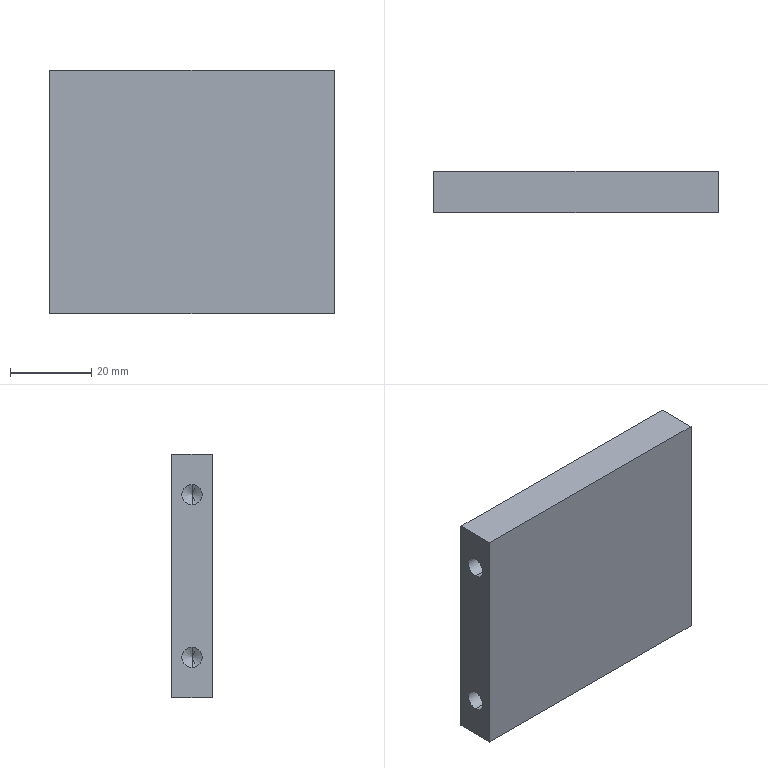Part | STEP file | Tube support mounting bracket upright plate | 1 solid | 22 faces | box 70 x 10 x 60 mm | volume 40154 mm3 | cylinder 8 | cone 8 | plane 6 | commonest cylinder face diameters 5 x8
STEP:
#1=CARTESIAN_POINT('',(0.,0.,0.));
#2=DIRECTION('',(0.,0.,1.));
#3=DIRECTION('',(1.,0.,0.));
#4=AXIS2_PLACEMENT_3D('',#1,#2,#3);
#5=CARTESIAN_POINT('',(-12.,0.,22.5));
#6=VERTEX_POINT('',#5);
#7=CARTESIAN_POINT('',(-35.,0.,22.5));
#8=VERTEX_POINT('',#7);
#9=CARTESIAN_POINT('',(-35.,0.,22.5));
#10=DIRECTION('',(-1.,0.,0.));
#11=VECTOR('',#10,1.);
#12=LINE('',#9,#11);
#13=CARTESIAN_POINT('',(-35.,0.,20.));
#14=DIRECTION('',(-1.,0.,0.));
#15=DIRECTION('',(0.,0.,1.));
#16=AXIS2_PLACEMENT_3D('',#13,#14,#15);
#17=CYLINDRICAL_SURFACE('',#16,2.5);
#18=CARTESIAN_POINT('',(6.283,0.));
#19=DIRECTION('',(0.,1.));
#20=VECTOR('',#19,1.);
#21=LINE('',#18,#20);
#22=(GEOMETRIC_REPRESENTATION_CONTEXT(2)PARAMETRIC_REPRESENTATION_CONTEXT()REPRESENTATION_CONTEXT('',''));
#23=DEFINITIONAL_REPRESENTATION('',(#21),#22);
#24=PCURVE('',#17,#23);
#25=CARTESIAN_POINT('',(-35.,0.,20.));
#26=DIRECTION('',(-1.,0.,0.));
#27=DIRECTION('',(0.,0.,1.));
#28=AXIS2_PLACEMENT_3D('',#25,#26,#27);
#29=CYLINDRICAL_SURFACE('',#28,2.5);
#30=CARTESIAN_POINT('',(0.,0.));
#31=DIRECTION('',(0.,1.));
#32=VECTOR('',#31,1.);
#33=LINE('',#30,#32);
#34=(GEOMETRIC_REPRESENTATION_CONTEXT(2)PARAMETRIC_REPRESENTATION_CONTEXT()REPRESENTATION_CONTEXT('',''));
#35=DEFINITIONAL_REPRESENTATION('',(#33),#34);
#36=PCURVE('',#29,#35);
#37=SURFACE_CURVE('',#12,(#24,#36),.PCURVE_S1.);
#38=EDGE_CURVE('',#6,#8,#37,.T.);
#39=ORIENTED_EDGE('',*,*,#38,.T.);
#40=CARTESIAN_POINT('',(-35.,0.,17.5));
#41=VERTEX_POINT('',#40);
#42=CARTESIAN_POINT('',(-35.,0.,20.));
#43=DIRECTION('',(-1.,0.,0.));
#44=DIRECTION('',(0.,0.,1.));
#45=AXIS2_PLACEMENT_3D('',#42,#43,#44);
#46=CIRCLE('',#45,2.5);
#47=CARTESIAN_POINT('',(0.,0.));
#48=DIRECTION('',(1.,0.));
#49=VECTOR('',#48,1.);
#50=LINE('',#47,#49);
#51=(GEOMETRIC_REPRESENTATION_CONTEXT(2)PARAMETRIC_REPRESENTATION_CONTEXT()REPRESENTATION_CONTEXT('',''));
#52=DEFINITIONAL_REPRESENTATION('',(#50),#51);
#53=PCURVE('',#17,#52);
#54=CARTESIAN_POINT('',(-35.,5.,30.));
#55=DIRECTION('',(1.,0.,0.));
#56=DIRECTION('',(0.,0.,-1.));
#57=AXIS2_PLACEMENT_3D('',#54,#55,#56);
#58=PLANE('',#57);
#59=CARTESIAN_POINT('',(7.5,-5.));
#60=CARTESIAN_POINT('',(7.5,-0.6699));
#61=CARTESIAN_POINT('',(11.25,-2.835));
#62=CARTESIAN_POINT('',(15.,-5.));
#63=CARTESIAN_POINT('',(11.25,-7.165));
#64=CARTESIAN_POINT('',(7.5,-9.33));
#65=CARTESIAN_POINT('',(7.5,-5.));
#66=(BOUNDED_CURVE()B_SPLINE_CURVE(2,(#59,#60,#61,#62,#63,#64,#65),.UNSPECIFIED.,.T.,.F.)B_SPLINE_CURVE_WITH_KNOTS((1,2,2,2,2,1),(-2.094,0.,2.094,4.189,6.283,8.378),.UNSPECIFIED.)CURVE()GEOMETRIC_REPRESENTATION_ITEM()RATIONAL_B_SPLINE_CURVE((1.,0.5,1.,0.5,1.,0.5,1.))REPRESENTATION_ITEM(''));
#67=(GEOMETRIC_REPRESENTATION_CONTEXT(2)PARAMETRIC_REPRESENTATION_CONTEXT()REPRESENTATION_CONTEXT('',''));
#68=DEFINITIONAL_REPRESENTATION('',(#66),#67);
#69=PCURVE('',#58,#68);
#70=SURFACE_CURVE('',#46,(#53,#69),.PCURVE_S1.);
#71=EDGE_CURVE('',#41,#8,#70,.T.);
#72=ORIENTED_EDGE('',*,*,#71,.F.);
#73=CARTESIAN_POINT('',(-12.,0.,17.5));
#74=VERTEX_POINT('',#73);
#75=CARTESIAN_POINT('',(-35.,0.,17.5));
#76=DIRECTION('',(-1.,0.,0.));
#77=VECTOR('',#76,1.);
#78=LINE('',#75,#77);
#79=CARTESIAN_POINT('',(3.142,0.));
#80=DIRECTION('',(0.,1.));
#81=VECTOR('',#80,1.);
#82=LINE('',#79,#81);
#83=(GEOMETRIC_REPRESENTATION_CONTEXT(2)PARAMETRIC_REPRESENTATION_CONTEXT()REPRESENTATION_CONTEXT('',''));
#84=DEFINITIONAL_REPRESENTATION('',(#82),#83);
#85=PCURVE('',#17,#84);
#86=CARTESIAN_POINT('',(3.142,0.));
#87=DIRECTION('',(0.,1.));
#88=VECTOR('',#87,1.);
#89=LINE('',#86,#88);
#90=(GEOMETRIC_REPRESENTATION_CONTEXT(2)PARAMETRIC_REPRESENTATION_CONTEXT()REPRESENTATION_CONTEXT('',''));
#91=DEFINITIONAL_REPRESENTATION('',(#89),#90);
#92=PCURVE('',#29,#91);
#93=SURFACE_CURVE('',#78,(#85,#92),.PCURVE_S1.);
#94=EDGE_CURVE('',#74,#41,#93,.T.);
#95=ORIENTED_EDGE('',*,*,#94,.F.);
#96=CARTESIAN_POINT('',(-12.,0.,20.));
#97=DIRECTION('',(-1.,0.,0.));
#98=DIRECTION('',(0.,0.,1.));
#99=AXIS2_PLACEMENT_3D('',#96,#97,#98);
#100=CIRCLE('',#99,2.5);
#101=CARTESIAN_POINT('',(0.,-23.));
#102=DIRECTION('',(1.,0.));
#103=VECTOR('',#102,1.);
#104=LINE('',#101,#103);
#105=(GEOMETRIC_REPRESENTATION_CONTEXT(2)PARAMETRIC_REPRESENTATION_CONTEXT()REPRESENTATION_CONTEXT('',''));
#106=DEFINITIONAL_REPRESENTATION('',(#104),#105);
#107=PCURVE('',#17,#106);
#108=CARTESIAN_POINT('',(-12.,0.,20.));
#109=DIRECTION('',(-1.,0.,0.));
#110=DIRECTION('',(0.,0.,1.));
#111=AXIS2_PLACEMENT_3D('',#108,#109,#110);
#112=CONICAL_SURFACE('',#111,2.5,1.03);
#113=CARTESIAN_POINT('',(0.,0.));
#114=DIRECTION('',(1.,0.));
#115=VECTOR('',#114,1.);
#116=LINE('',#113,#115);
#117=(GEOMETRIC_REPRESENTATION_CONTEXT(2)PARAMETRIC_REPRESENTATION_CONTEXT()REPRESENTATION_CONTEXT('',''));
#118=DEFINITIONAL_REPRESENTATION('',(#116),#117);
#119=PCURVE('',#112,#118);
#120=SURFACE_CURVE('',#100,(#107,#119),.PCURVE_S1.);
#121=EDGE_CURVE('',#74,#6,#120,.T.);
#122=ORIENTED_EDGE('',*,*,#121,.T.);
#123=EDGE_LOOP('',(#39,#72,#95,#122));
#124=FACE_BOUND('',#123,.F.);
#125=ADVANCED_FACE('',(#124),#17,.F.);
#126=ORIENTED_EDGE('',*,*,#121,.F.);
#127=CARTESIAN_POINT('',(-10.498,0.,20.));
#128=VERTEX_POINT('',#127);
#129=CARTESIAN_POINT('',(-12.,0.,17.5));
#130=DIRECTION('',(-0.515,0.,-0.8572));
#131=VECTOR('',#130,1.);
#132=LINE('',#129,#131);
#133=CARTESIAN_POINT('',(3.142,0.));
#134=DIRECTION('',(0.,1.));
#135=VECTOR('',#134,1.);
#136=LINE('',#133,#135);
#137=(GEOMETRIC_REPRESENTATION_CONTEXT(2)PARAMETRIC_REPRESENTATION_CONTEXT()REPRESENTATION_CONTEXT('',''));
#138=DEFINITIONAL_REPRESENTATION('',(#136),#137);
#139=PCURVE('',#112,#138);
#140=CARTESIAN_POINT('',(-12.,0.,20.));
#141=DIRECTION('',(-1.,0.,0.));
#142=DIRECTION('',(0.,0.,1.));
#143=AXIS2_PLACEMENT_3D('',#140,#141,#142);
#144=CONICAL_SURFACE('',#143,2.5,1.03);
#145=CARTESIAN_POINT('',(3.142,0.));
#146=DIRECTION('',(0.,1.));
#147=VECTOR('',#146,1.);
#148=LINE('',#145,#147);
#149=(GEOMETRIC_REPRESENTATION_CONTEXT(2)PARAMETRIC_REPRESENTATION_CONTEXT()REPRESENTATION_CONTEXT('',''));
#150=DEFINITIONAL_REPRESENTATION('',(#148),#149);
#151=PCURVE('',#144,#150);
#152=SURFACE_CURVE('',#132,(#139,#151),.PCURVE_S1.);
#153=EDGE_CURVE('',#128,#74,#152,.T.);
#154=ORIENTED_EDGE('',*,*,#153,.F.);
#155=CARTESIAN_POINT('',(-12.,0.,22.5));
#156=DIRECTION('',(-0.515,0.,0.8572));
#157=VECTOR('',#156,1.);
#158=LINE('',#155,#157);
#159=CARTESIAN_POINT('',(6.283,0.));
#160=DIRECTION('',(0.,1.));
#161=VECTOR('',#160,1.);
#162=LINE('',#159,#161);
#163=(GEOMETRIC_REPRESENTATION_CONTEXT(2)PARAMETRIC_REPRESENTATION_CONTEXT()REPRESENTATION_CONTEXT('',''));
#164=DEFINITIONAL_REPRESENTATION('',(#162),#163);
#165=PCURVE('',#112,#164);
#166=CARTESIAN_POINT('',(0.,0.));
#167=DIRECTION('',(0.,1.));
#168=VECTOR('',#167,1.);
#169=LINE('',#166,#168);
#170=(GEOMETRIC_REPRESENTATION_CONTEXT(2)PARAMETRIC_REPRESENTATION_CONTEXT()REPRESENTATION_CONTEXT('',''));
#171=DEFINITIONAL_REPRESENTATION('',(#169),#170);
#172=PCURVE('',#144,#171);
#173=SURFACE_CURVE('',#158,(#165,#172),.PCURVE_S1.);
#174=EDGE_CURVE('',#128,#6,#173,.T.);
#175=ORIENTED_EDGE('',*,*,#174,.T.);
#176=EDGE_LOOP('',(#126,#154,#175));
#177=FACE_BOUND('',#176,.F.);
#178=ADVANCED_FACE('',(#177),#112,.F.);
#179=CARTESIAN_POINT('',(-12.,0.,-17.5));
#180=VERTEX_POINT('',#179);
#181=CARTESIAN_POINT('',(-35.,0.,-17.5));
#182=VERTEX_POINT('',#181);
#183=CARTESIAN_POINT('',(-35.,0.,-17.5));
#184=DIRECTION('',(-1.,0.,0.));
#185=VECTOR('',#184,1.);
#186=LINE('',#183,#185);
#187=CARTESIAN_POINT('',(-35.,0.,-20.));
#188=DIRECTION('',(-1.,0.,0.));
#189=DIRECTION('',(0.,0.,1.));
#190=AXIS2_PLACEMENT_3D('',#187,#188,#189);
#191=CYLINDRICAL_SURFACE('',#190,2.5);
#192=CARTESIAN_POINT('',(6.283,0.));
#193=DIRECTION('',(0.,1.));
#194=VECTOR('',#193,1.);
#195=LINE('',#192,#194);
#196=(GEOMETRIC_REPRESENTATION_CONTEXT(2)PARAMETRIC_REPRESENTATION_CONTEXT()REPRESENTATION_CONTEXT('',''));
#197=DEFINITIONAL_REPRESENTATION('',(#195),#196);
#198=PCURVE('',#191,#197);
#199=CARTESIAN_POINT('',(-35.,0.,-20.));
#200=DIRECTION('',(-1.,0.,0.));
#201=DIRECTION('',(0.,0.,1.));
#202=AXIS2_PLACEMENT_3D('',#199,#200,#201);
#203=CYLINDRICAL_SURFACE('',#202,2.5);
#204=CARTESIAN_POINT('',(0.,0.));
#205=DIRECTION('',(0.,1.));
#206=VECTOR('',#205,1.);
#207=LINE('',#204,#206);
#208=(GEOMETRIC_REPRESENTATION_CONTEXT(2)PARAMETRIC_REPRESENTATION_CONTEXT()REPRESENTATION_CONTEXT('',''));
#209=DEFINITIONAL_REPRESENTATION('',(#207),#208);
#210=PCURVE('',#203,#209);
#211=SURFACE_CURVE('',#186,(#198,#210),.PCURVE_S1.);
#212=EDGE_CURVE('',#180,#182,#211,.T.);
#213=ORIENTED_EDGE('',*,*,#212,.T.);
#214=CARTESIAN_POINT('',(-35.,0.,-22.5));
#215=VERTEX_POINT('',#214);
#216=CARTESIAN_POINT('',(-35.,0.,-20.));
#217=DIRECTION('',(-1.,0.,0.));
#218=DIRECTION('',(0.,0.,1.));
#219=AXIS2_PLACEMENT_3D('',#216,#217,#218);
#220=CIRCLE('',#219,2.5);
#221=CARTESIAN_POINT('',(0.,0.));
#222=DIRECTION('',(1.,0.));
#223=VECTOR('',#222,1.);
#224=LINE('',#221,#223);
#225=(GEOMETRIC_REPRESENTATION_CONTEXT(2)PARAMETRIC_REPRESENTATION_CONTEXT()REPRESENTATION_CONTEXT('',''));
#226=DEFINITIONAL_REPRESENTATION('',(#224),#225);
#227=PCURVE('',#191,#226);
#228=CARTESIAN_POINT('',(47.5,-5.));
#229=CARTESIAN_POINT('',(47.5,-0.6699));
#230=CARTESIAN_POINT('',(51.25,-2.835));
#231=CARTESIAN_POINT('',(55.,-5.));
#232=CARTESIAN_POINT('',(51.25,-7.165));
#233=CARTESIAN_POINT('',(47.5,-9.33));
#234=CARTESIAN_POINT('',(47.5,-5.));
#235=(BOUNDED_CURVE()B_SPLINE_CURVE(2,(#228,#229,#230,#231,#232,#233,#234),.UNSPECIFIED.,.T.,.F.)B_SPLINE_CURVE_WITH_KNOTS((1,2,2,2,2,1),(-2.094,0.,2.094,4.189,6.283,8.378),.UNSPECIFIED.)CURVE()GEOMETRIC_REPRESENTATION_ITEM()RATIONAL_B_SPLINE_CURVE((1.,0.5,1.,0.5,1.,0.5,1.))REPRESENTATION_ITEM(''));
#236=(GEOMETRIC_REPRESENTATION_CONTEXT(2)PARAMETRIC_REPRESENTATION_CONTEXT()REPRESENTATION_CONTEXT('',''));
#237=DEFINITIONAL_REPRESENTATION('',(#235),#236);
#238=PCURVE('',#58,#237);
#239=SURFACE_CURVE('',#220,(#227,#238),.PCURVE_S1.);
#240=EDGE_CURVE('',#215,#182,#239,.T.);
#241=ORIENTED_EDGE('',*,*,#240,.F.);
#242=CARTESIAN_POINT('',(-12.,0.,-22.5));
#243=VERTEX_POINT('',#242);
#244=CARTESIAN_POINT('',(-35.,0.,-22.5));
#245=DIRECTION('',(-1.,0.,0.));
#246=VECTOR('',#245,1.);
#247=LINE('',#244,#246);
#248=CARTESIAN_POINT('',(3.142,0.));
#249=DIRECTION('',(0.,1.));
#250=VECTOR('',#249,1.);
#251=LINE('',#248,#250);
#252=(GEOMETRIC_REPRESENTATION_CONTEXT(2)PARAMETRIC_REPRESENTATION_CONTEXT()REPRESENTATION_CONTEXT('',''));
#253=DEFINITIONAL_REPRESENTATION('',(#251),#252);
#254=PCURVE('',#191,#253);
#255=CARTESIAN_POINT('',(3.142,0.));
#256=DIRECTION('',(0.,1.));
#257=VECTOR('',#256,1.);
#258=LINE('',#255,#257);
#259=(GEOMETRIC_REPRESENTATION_CONTEXT(2)PARAMETRIC_REPRESENTATION_CONTEXT()REPRESENTATION_CONTEXT('',''));
#260=DEFINITIONAL_REPRESENTATION('',(#258),#259);
#261=PCURVE('',#203,#260);
#262=SURFACE_CURVE('',#247,(#254,#261),.PCURVE_S1.);
#263=EDGE_CURVE('',#243,#215,#262,.T.);
#264=ORIENTED_EDGE('',*,*,#263,.F.);
#265=CARTESIAN_POINT('',(-12.,0.,-20.));
#266=DIRECTION('',(-1.,0.,0.));
#267=DIRECTION('',(0.,0.,1.));
#268=AXIS2_PLACEMENT_3D('',#265,#266,#267);
#269=CIRCLE('',#268,2.5);
#270=CARTESIAN_POINT('',(0.,-23.));
#271=DIRECTION('',(1.,0.));
#272=VECTOR('',#271,1.);
#273=LINE('',#270,#272);
#274=(GEOMETRIC_REPRESENTATION_CONTEXT(2)PARAMETRIC_REPRESENTATION_CONTEXT()REPRESENTATION_CONTEXT('',''));
#275=DEFINITIONAL_REPRESENTATION('',(#273),#274);
#276=PCURVE('',#191,#275);
#277=CARTESIAN_POINT('',(-12.,0.,-20.));
#278=DIRECTION('',(-1.,0.,0.));
#279=DIRECTION('',(0.,0.,1.));
#280=AXIS2_PLACEMENT_3D('',#277,#278,#279);
#281=CONICAL_SURFACE('',#280,2.5,1.03);
#282=CARTESIAN_POINT('',(0.,0.));
#283=DIRECTION('',(1.,0.));
#284=VECTOR('',#283,1.);
#285=LINE('',#282,#284);
#286=(GEOMETRIC_REPRESENTATION_CONTEXT(2)PARAMETRIC_REPRESENTATION_CONTEXT()REPRESENTATION_CONTEXT('',''));
#287=DEFINITIONAL_REPRESENTATION('',(#285),#286);
#288=PCURVE('',#281,#287);
#289=SURFACE_CURVE('',#269,(#276,#288),.PCURVE_S1.);
#290=EDGE_CURVE('',#243,#180,#289,.T.);
#291=ORIENTED_EDGE('',*,*,#290,.T.);
#292=EDGE_LOOP('',(#213,#241,#264,#291));
#293=FACE_BOUND('',#292,.F.);
#294=ADVANCED_FACE('',(#293),#191,.F.);
#295=ORIENTED_EDGE('',*,*,#290,.F.);
#296=CARTESIAN_POINT('',(-10.498,0.,-20.));
#297=VERTEX_POINT('',#296);
#298=CARTESIAN_POINT('',(-12.,0.,-22.5));
#299=DIRECTION('',(-0.515,0.,-0.8572));
#300=VECTOR('',#299,1.);
#301=LINE('',#298,#300);
#302=CARTESIAN_POINT('',(3.142,0.));
#303=DIRECTION('',(0.,1.));
#304=VECTOR('',#303,1.);
#305=LINE('',#302,#304);
#306=(GEOMETRIC_REPRESENTATION_CONTEXT(2)PARAMETRIC_REPRESENTATION_CONTEXT()REPRESENTATION_CONTEXT('',''));
#307=DEFINITIONAL_REPRESENTATION('',(#305),#306);
#308=PCURVE('',#281,#307);
#309=CARTESIAN_POINT('',(-12.,0.,-20.));
#310=DIRECTION('',(-1.,0.,0.));
#311=DIRECTION('',(0.,0.,1.));
#312=AXIS2_PLACEMENT_3D('',#309,#310,#311);
#313=CONICAL_SURFACE('',#312,2.5,1.03);
#314=CARTESIAN_POINT('',(3.142,0.));
#315=DIRECTION('',(0.,1.));
#316=VECTOR('',#315,1.);
#317=LINE('',#314,#316);
#318=(GEOMETRIC_REPRESENTATION_CONTEXT(2)PARAMETRIC_REPRESENTATION_CONTEXT()REPRESENTATION_CONTEXT('',''));
#319=DEFINITIONAL_REPRESENTATION('',(#317),#318);
#320=PCURVE('',#313,#319);
#321=SURFACE_CURVE('',#301,(#308,#320),.PCURVE_S1.);
#322=EDGE_CURVE('',#297,#243,#321,.T.);
#323=ORIENTED_EDGE('',*,*,#322,.F.);
#324=CARTESIAN_POINT('',(-12.,0.,-17.5));
#325=DIRECTION('',(-0.515,0.,0.8572));
#326=VECTOR('',#325,1.);
#327=LINE('',#324,#326);
#328=CARTESIAN_POINT('',(6.283,0.));
#329=DIRECTION('',(0.,1.));
#330=VECTOR('',#329,1.);
#331=LINE('',#328,#330);
#332=(GEOMETRIC_REPRESENTATION_CONTEXT(2)PARAMETRIC_REPRESENTATION_CONTEXT()REPRESENTATION_CONTEXT('',''));
#333=DEFINITIONAL_REPRESENTATION('',(#331),#332);
#334=PCURVE('',#281,#333);
#335=CARTESIAN_POINT('',(0.,0.));
#336=DIRECTION('',(0.,1.));
#337=VECTOR('',#336,1.);
#338=LINE('',#335,#337);
#339=(GEOMETRIC_REPRESENTATION_CONTEXT(2)PARAMETRIC_REPRESENTATION_CONTEXT()REPRESENTATION_CONTEXT('',''));
#340=DEFINITIONAL_REPRESENTATION('',(#338),#339);
#341=PCURVE('',#313,#340);
#342=SURFACE_CURVE('',#327,(#334,#341),.PCURVE_S1.);
#343=EDGE_CURVE('',#297,#180,#342,.T.);
#344=ORIENTED_EDGE('',*,*,#343,.T.);
#345=EDGE_LOOP('',(#295,#323,#344));
#346=FACE_BOUND('',#345,.F.);
#347=ADVANCED_FACE('',(#346),#281,.F.);
#348=CARTESIAN_POINT('',(12.,0.,17.5));
#349=VERTEX_POINT('',#348);
#350=CARTESIAN_POINT('',(35.,0.,17.5));
#351=VERTEX_POINT('',#350);
#352=CARTESIAN_POINT('',(35.,0.,17.5));
#353=DIRECTION('',(1.,0.,0.));
#354=VECTOR('',#353,1.);
#355=LINE('',#352,#354);
#356=CARTESIAN_POINT('',(35.,0.,20.));
#357=DIRECTION('',(1.,0.,0.));
#358=DIRECTION('',(0.,0.,-1.));
#359=AXIS2_PLACEMENT_3D('',#356,#357,#358);
#360=CYLINDRICAL_SURFACE('',#359,2.5);
#361=CARTESIAN_POINT('',(6.283,0.));
#362=DIRECTION('',(0.,1.));
#363=VECTOR('',#362,1.);
#364=LINE('',#361,#363);
#365=(GEOMETRIC_REPRESENTATION_CONTEXT(2)PARAMETRIC_REPRESENTATION_CONTEXT()REPRESENTATION_CONTEXT('',''));
#366=DEFINITIONAL_REPRESENTATION('',(#364),#365);
#367=PCURVE('',#360,#366);
#368=CARTESIAN_POINT('',(35.,0.,20.));
#369=DIRECTION('',(1.,0.,0.));
#370=DIRECTION('',(0.,0.,-1.));
#371=AXIS2_PLACEMENT_3D('',#368,#369,#370);
#372=CYLINDRICAL_SURFACE('',#371,2.5);
#373=CARTESIAN_POINT('',(0.,0.));
#374=DIRECTION('',(0.,1.));
#375=VECTOR('',#374,1.);
#376=LINE('',#373,#375);
#377=(GEOMETRIC_REPRESENTATION_CONTEXT(2)PARAMETRIC_REPRESENTATION_CONTEXT()REPRESENTATION_CONTEXT('',''));
#378=DEFINITIONAL_REPRESENTATION('',(#376),#377);
#379=PCURVE('',#372,#378);
#380=SURFACE_CURVE('',#355,(#367,#379),.PCURVE_S1.);
#381=EDGE_CURVE('',#349,#351,#380,.T.);
#382=ORIENTED_EDGE('',*,*,#381,.T.);
#383=CARTESIAN_POINT('',(35.,0.,22.5));
#384=VERTEX_POINT('',#383);
#385=CARTESIAN_POINT('',(35.,0.,20.));
#386=DIRECTION('',(1.,0.,0.));
#387=DIRECTION('',(0.,0.,-1.));
#388=AXIS2_PLACEMENT_3D('',#385,#386,#387);
#389=CIRCLE('',#388,2.5);
#390=CARTESIAN_POINT('',(0.,0.));
#391=DIRECTION('',(1.,0.));
#392=VECTOR('',#391,1.);
#393=LINE('',#390,#392);
#394=(GEOMETRIC_REPRESENTATION_CONTEXT(2)PARAMETRIC_REPRESENTATION_CONTEXT()REPRESENTATION_CONTEXT('',''));
#395=DEFINITIONAL_REPRESENTATION('',(#393),#394);
#396=PCURVE('',#360,#395);
#397=CARTESIAN_POINT('',(35.,5.,30.));
#398=DIRECTION('',(-1.,0.,0.));
#399=DIRECTION('',(0.,0.,1.));
#400=AXIS2_PLACEMENT_3D('',#397,#398,#399);
#401=PLANE('',#400);
#402=CARTESIAN_POINT('',(-12.5,-5.));
#403=CARTESIAN_POINT('',(-12.5,-0.6699));
#404=CARTESIAN_POINT('',(-8.75,-2.835));
#405=CARTESIAN_POINT('',(-5.,-5.));
#406=CARTESIAN_POINT('',(-8.75,-7.165));
#407=CARTESIAN_POINT('',(-12.5,-9.33));
#408=CARTESIAN_POINT('',(-12.5,-5.));
#409=(BOUNDED_CURVE()B_SPLINE_CURVE(2,(#402,#403,#404,#405,#406,#407,#408),.UNSPECIFIED.,.T.,.F.)B_SPLINE_CURVE_WITH_KNOTS((1,2,2,2,2,1),(-2.094,0.,2.094,4.189,6.283,8.378),.UNSPECIFIED.)CURVE()GEOMETRIC_REPRESENTATION_ITEM()RATIONAL_B_SPLINE_CURVE((1.,0.5,1.,0.5,1.,0.5,1.))REPRESENTATION_ITEM(''));
#410=(GEOMETRIC_REPRESENTATION_CONTEXT(2)PARAMETRIC_REPRESENTATION_CONTEXT()REPRESENTATION_CONTEXT('',''));
#411=DEFINITIONAL_REPRESENTATION('',(#409),#410);
#412=PCURVE('',#401,#411);
#413=SURFACE_CURVE('',#389,(#396,#412),.PCURVE_S1.);
#414=EDGE_CURVE('',#384,#351,#413,.T.);
#415=ORIENTED_EDGE('',*,*,#414,.F.);
#416=CARTESIAN_POINT('',(12.,0.,22.5));
#417=VERTEX_POINT('',#416);
#418=CARTESIAN_POINT('',(35.,0.,22.5));
#419=DIRECTION('',(1.,0.,0.));
#420=VECTOR('',#419,1.);
#421=LINE('',#418,#420);
#422=CARTESIAN_POINT('',(3.142,0.));
#423=DIRECTION('',(0.,1.));
#424=VECTOR('',#423,1.);
#425=LINE('',#422,#424);
#426=(GEOMETRIC_REPRESENTATION_CONTEXT(2)PARAMETRIC_REPRESENTATION_CONTEXT()REPRESENTATION_CONTEXT('',''));
#427=DEFINITIONAL_REPRESENTATION('',(#425),#426);
#428=PCURVE('',#360,#427);
#429=CARTESIAN_POINT('',(3.142,0.));
#430=DIRECTION('',(0.,1.));
#431=VECTOR('',#430,1.);
#432=LINE('',#429,#431);
#433=(GEOMETRIC_REPRESENTATION_CONTEXT(2)PARAMETRIC_REPRESENTATION_CONTEXT()REPRESENTATION_CONTEXT('',''));
#434=DEFINITIONAL_REPRESENTATION('',(#432),#433);
#435=PCURVE('',#372,#434);
#436=SURFACE_CURVE('',#421,(#428,#435),.PCURVE_S1.);
#437=EDGE_CURVE('',#417,#384,#436,.T.);
#438=ORIENTED_EDGE('',*,*,#437,.F.);
#439=CARTESIAN_POINT('',(12.,0.,20.));
#440=DIRECTION('',(1.,0.,0.));
#441=DIRECTION('',(0.,0.,-1.));
#442=AXIS2_PLACEMENT_3D('',#439,#440,#441);
#443=CIRCLE('',#442,2.5);
#444=CARTESIAN_POINT('',(0.,-23.));
#445=DIRECTION('',(1.,0.));
#446=VECTOR('',#445,1.);
#447=LINE('',#444,#446);
#448=(GEOMETRIC_REPRESENTATION_CONTEXT(2)PARAMETRIC_REPRESENTATION_CONTEXT()REPRESENTATION_CONTEXT('',''));
#449=DEFINITIONAL_REPRESENTATION('',(#447),#448);
#450=PCURVE('',#360,#449);
#451=CARTESIAN_POINT('',(12.,0.,20.));
#452=DIRECTION('',(1.,0.,0.));
#453=DIRECTION('',(0.,0.,-1.));
#454=AXIS2_PLACEMENT_3D('',#451,#452,#453);
#455=CONICAL_SURFACE('',#454,2.5,1.03);
#456=CARTESIAN_POINT('',(0.,0.));
#457=DIRECTION('',(1.,0.));
#458=VECTOR('',#457,1.);
#459=LINE('',#456,#458);
#460=(GEOMETRIC_REPRESENTATION_CONTEXT(2)PARAMETRIC_REPRESENTATION_CONTEXT()REPRESENTATION_CONTEXT('',''));
#461=DEFINITIONAL_REPRESENTATION('',(#459),#460);
#462=PCURVE('',#455,#461);
#463=SURFACE_CURVE('',#443,(#450,#462),.PCURVE_S1.);
#464=EDGE_CURVE('',#417,#349,#463,.T.);
#465=ORIENTED_EDGE('',*,*,#464,.T.);
#466=EDGE_LOOP('',(#382,#415,#438,#465));
#467=FACE_BOUND('',#466,.F.);
#468=ADVANCED_FACE('',(#467),#360,.F.);
#469=ORIENTED_EDGE('',*,*,#464,.F.);
#470=CARTESIAN_POINT('',(10.498,0.,20.));
#471=VERTEX_POINT('',#470);
#472=CARTESIAN_POINT('',(12.,0.,22.5));
#473=DIRECTION('',(0.515,0.,0.8572));
#474=VECTOR('',#473,1.);
#475=LINE('',#472,#474);
#476=CARTESIAN_POINT('',(3.142,0.));
#477=DIRECTION('',(0.,1.));
#478=VECTOR('',#477,1.);
#479=LINE('',#476,#478);
#480=(GEOMETRIC_REPRESENTATION_CONTEXT(2)PARAMETRIC_REPRESENTATION_CONTEXT()REPRESENTATION_CONTEXT('',''));
#481=DEFINITIONAL_REPRESENTATION('',(#479),#480);
#482=PCURVE('',#455,#481);
#483=CARTESIAN_POINT('',(12.,0.,20.));
#484=DIRECTION('',(1.,0.,0.));
#485=DIRECTION('',(0.,0.,-1.));
#486=AXIS2_PLACEMENT_3D('',#483,#484,#485);
#487=CONICAL_SURFACE('',#486,2.5,1.03);
#488=CARTESIAN_POINT('',(3.142,0.));
#489=DIRECTION('',(0.,1.));
#490=VECTOR('',#489,1.);
#491=LINE('',#488,#490);
#492=(GEOMETRIC_REPRESENTATION_CONTEXT(2)PARAMETRIC_REPRESENTATION_CONTEXT()REPRESENTATION_CONTEXT('',''));
#493=DEFINITIONAL_REPRESENTATION('',(#491),#492);
#494=PCURVE('',#487,#493);
#495=SURFACE_CURVE('',#475,(#482,#494),.PCURVE_S1.);
#496=EDGE_CURVE('',#471,#417,#495,.T.);
#497=ORIENTED_EDGE('',*,*,#496,.F.);
#498=CARTESIAN_POINT('',(12.,0.,17.5));
#499=DIRECTION('',(0.515,0.,-0.8572));
#500=VECTOR('',#499,1.);
#501=LINE('',#498,#500);
#502=CARTESIAN_POINT('',(6.283,0.));
#503=DIRECTION('',(0.,1.));
#504=VECTOR('',#503,1.);
#505=LINE('',#502,#504);
#506=(GEOMETRIC_REPRESENTATION_CONTEXT(2)PARAMETRIC_REPRESENTATION_CONTEXT()REPRESENTATION_CONTEXT('',''));
#507=DEFINITIONAL_REPRESENTATION('',(#505),#506);
#508=PCURVE('',#455,#507);
#509=CARTESIAN_POINT('',(0.,0.));
#510=DIRECTION('',(0.,1.));
#511=VECTOR('',#510,1.);
#512=LINE('',#509,#511);
#513=(GEOMETRIC_REPRESENTATION_CONTEXT(2)PARAMETRIC_REPRESENTATION_CONTEXT()REPRESENTATION_CONTEXT('',''));
#514=DEFINITIONAL_REPRESENTATION('',(#512),#513);
#515=PCURVE('',#487,#514);
#516=SURFACE_CURVE('',#501,(#508,#515),.PCURVE_S1.);
#517=EDGE_CURVE('',#471,#349,#516,.T.);
#518=ORIENTED_EDGE('',*,*,#517,.T.);
#519=EDGE_LOOP('',(#469,#497,#518));
#520=FACE_BOUND('',#519,.F.);
#521=ADVANCED_FACE('',(#520),#455,.F.);
#522=CARTESIAN_POINT('',(12.,0.,-22.5));
#523=VERTEX_POINT('',#522);
#524=CARTESIAN_POINT('',(35.,0.,-22.5));
#525=VERTEX_POINT('',#524);
#526=CARTESIAN_POINT('',(35.,0.,-22.5));
#527=DIRECTION('',(1.,0.,0.));
#528=VECTOR('',#527,1.);
#529=LINE('',#526,#528);
#530=CARTESIAN_POINT('',(35.,0.,-20.));
#531=DIRECTION('',(1.,0.,0.));
#532=DIRECTION('',(0.,0.,-1.));
#533=AXIS2_PLACEMENT_3D('',#530,#531,#532);
#534=CYLINDRICAL_SURFACE('',#533,2.5);
#535=CARTESIAN_POINT('',(6.283,0.));
#536=DIRECTION('',(0.,1.));
#537=VECTOR('',#536,1.);
#538=LINE('',#535,#537);
#539=(GEOMETRIC_REPRESENTATION_CONTEXT(2)PARAMETRIC_REPRESENTATION_CONTEXT()REPRESENTATION_CONTEXT('',''));
#540=DEFINITIONAL_REPRESENTATION('',(#538),#539);
#541=PCURVE('',#534,#540);
#542=CARTESIAN_POINT('',(35.,0.,-20.));
#543=DIRECTION('',(1.,0.,0.));
#544=DIRECTION('',(0.,0.,-1.));
#545=AXIS2_PLACEMENT_3D('',#542,#543,#544);
#546=CYLINDRICAL_SURFACE('',#545,2.5);
#547=CARTESIAN_POINT('',(0.,0.));
#548=DIRECTION('',(0.,1.));
#549=VECTOR('',#548,1.);
#550=LINE('',#547,#549);
#551=(GEOMETRIC_REPRESENTATION_CONTEXT(2)PARAMETRIC_REPRESENTATION_CONTEXT()REPRESENTATION_CONTEXT('',''));
#552=DEFINITIONAL_REPRESENTATION('',(#550),#551);
#553=PCURVE('',#546,#552);
#554=SURFACE_CURVE('',#529,(#541,#553),.PCURVE_S1.);
#555=EDGE_CURVE('',#523,#525,#554,.T.);
#556=ORIENTED_EDGE('',*,*,#555,.T.);
#557=CARTESIAN_POINT('',(35.,0.,-17.5));
#558=VERTEX_POINT('',#557);
#559=CARTESIAN_POINT('',(35.,0.,-20.));
#560=DIRECTION('',(1.,0.,0.));
#561=DIRECTION('',(0.,0.,-1.));
#562=AXIS2_PLACEMENT_3D('',#559,#560,#561);
#563=CIRCLE('',#562,2.5);
#564=CARTESIAN_POINT('',(0.,0.));
#565=DIRECTION('',(1.,0.));
#566=VECTOR('',#565,1.);
#567=LINE('',#564,#566);
#568=(GEOMETRIC_REPRESENTATION_CONTEXT(2)PARAMETRIC_REPRESENTATION_CONTEXT()REPRESENTATION_CONTEXT('',''));
#569=DEFINITIONAL_REPRESENTATION('',(#567),#568);
#570=PCURVE('',#534,#569);
#571=CARTESIAN_POINT('',(-52.5,-5.));
#572=CARTESIAN_POINT('',(-52.5,-0.6699));
#573=CARTESIAN_POINT('',(-48.75,-2.835));
#574=CARTESIAN_POINT('',(-45.,-5.));
#575=CARTESIAN_POINT('',(-48.75,-7.165));
#576=CARTESIAN_POINT('',(-52.5,-9.33));
#577=CARTESIAN_POINT('',(-52.5,-5.));
#578=(BOUNDED_CURVE()B_SPLINE_CURVE(2,(#571,#572,#573,#574,#575,#576,#577),.UNSPECIFIED.,.T.,.F.)B_SPLINE_CURVE_WITH_KNOTS((1,2,2,2,2,1),(-2.094,0.,2.094,4.189,6.283,8.378),.UNSPECIFIED.)CURVE()GEOMETRIC_REPRESENTATION_ITEM()RATIONAL_B_SPLINE_CURVE((1.,0.5,1.,0.5,1.,0.5,1.))REPRESENTATION_ITEM(''));
#579=(GEOMETRIC_REPRESENTATION_CONTEXT(2)PARAMETRIC_REPRESENTATION_CONTEXT()REPRESENTATION_CONTEXT('',''));
#580=DEFINITIONAL_REPRESENTATION('',(#578),#579);
#581=PCURVE('',#401,#580);
#582=SURFACE_CURVE('',#563,(#570,#581),.PCURVE_S1.);
#583=EDGE_CURVE('',#558,#525,#582,.T.);
#584=ORIENTED_EDGE('',*,*,#583,.F.);
#585=CARTESIAN_POINT('',(12.,0.,-17.5));
#586=VERTEX_POINT('',#585);
#587=CARTESIAN_POINT('',(35.,0.,-17.5));
#588=DIRECTION('',(1.,0.,0.));
#589=VECTOR('',#588,1.);
#590=LINE('',#587,#589);
#591=CARTESIAN_POINT('',(3.142,0.));
#592=DIRECTION('',(0.,1.));
#593=VECTOR('',#592,1.);
#594=LINE('',#591,#593);
#595=(GEOMETRIC_REPRESENTATION_CONTEXT(2)PARAMETRIC_REPRESENTATION_CONTEXT()REPRESENTATION_CONTEXT('',''));
#596=DEFINITIONAL_REPRESENTATION('',(#594),#595);
#597=PCURVE('',#534,#596);
#598=CARTESIAN_POINT('',(3.142,0.));
#599=DIRECTION('',(0.,1.));
#600=VECTOR('',#599,1.);
#601=LINE('',#598,#600);
#602=(GEOMETRIC_REPRESENTATION_CONTEXT(2)PARAMETRIC_REPRESENTATION_CONTEXT()REPRESENTATION_CONTEXT('',''));
#603=DEFINITIONAL_REPRESENTATION('',(#601),#602);
#604=PCURVE('',#546,#603);
#605=SURFACE_CURVE('',#590,(#597,#604),.PCURVE_S1.);
#606=EDGE_CURVE('',#586,#558,#605,.T.);
#607=ORIENTED_EDGE('',*,*,#606,.F.);
#608=CARTESIAN_POINT('',(12.,0.,-20.));
#609=DIRECTION('',(1.,0.,0.));
#610=DIRECTION('',(0.,0.,-1.));
#611=AXIS2_PLACEMENT_3D('',#608,#609,#610);
#612=CIRCLE('',#611,2.5);
#613=CARTESIAN_POINT('',(0.,-23.));
#614=DIRECTION('',(1.,0.));
#615=VECTOR('',#614,1.);
#616=LINE('',#613,#615);
#617=(GEOMETRIC_REPRESENTATION_CONTEXT(2)PARAMETRIC_REPRESENTATION_CONTEXT()REPRESENTATION_CONTEXT('',''));
#618=DEFINITIONAL_REPRESENTATION('',(#616),#617);
#619=PCURVE('',#534,#618);
#620=CARTESIAN_POINT('',(12.,0.,-20.));
#621=DIRECTION('',(1.,0.,0.));
#622=DIRECTION('',(0.,0.,-1.));
#623=AXIS2_PLACEMENT_3D('',#620,#621,#622);
#624=CONICAL_SURFACE('',#623,2.5,1.03);
#625=CARTESIAN_POINT('',(0.,0.));
#626=DIRECTION('',(1.,0.));
#627=VECTOR('',#626,1.);
#628=LINE('',#625,#627);
#629=(GEOMETRIC_REPRESENTATION_CONTEXT(2)PARAMETRIC_REPRESENTATION_CONTEXT()REPRESENTATION_CONTEXT('',''));
#630=DEFINITIONAL_REPRESENTATION('',(#628),#629);
#631=PCURVE('',#624,#630);
#632=SURFACE_CURVE('',#612,(#619,#631),.PCURVE_S1.);
#633=EDGE_CURVE('',#586,#523,#632,.T.);
#634=ORIENTED_EDGE('',*,*,#633,.T.);
#635=EDGE_LOOP('',(#556,#584,#607,#634));
#636=FACE_BOUND('',#635,.F.);
#637=ADVANCED_FACE('',(#636),#534,.F.);
#638=ORIENTED_EDGE('',*,*,#633,.F.);
#639=CARTESIAN_POINT('',(10.498,0.,-20.));
#640=VERTEX_POINT('',#639);
#641=CARTESIAN_POINT('',(12.,0.,-17.5));
#642=DIRECTION('',(0.515,0.,0.8572));
#643=VECTOR('',#642,1.);
#644=LINE('',#641,#643);
#645=CARTESIAN_POINT('',(3.142,0.));
#646=DIRECTION('',(0.,1.));
#647=VECTOR('',#646,1.);
#648=LINE('',#645,#647);
#649=(GEOMETRIC_REPRESENTATION_CONTEXT(2)PARAMETRIC_REPRESENTATION_CONTEXT()REPRESENTATION_CONTEXT('',''));
#650=DEFINITIONAL_REPRESENTATION('',(#648),#649);
#651=PCURVE('',#624,#650);
#652=CARTESIAN_POINT('',(12.,0.,-20.));
#653=DIRECTION('',(1.,0.,0.));
#654=DIRECTION('',(0.,0.,-1.));
#655=AXIS2_PLACEMENT_3D('',#652,#653,#654);
#656=CONICAL_SURFACE('',#655,2.5,1.03);
#657=CARTESIAN_POINT('',(3.142,0.));
#658=DIRECTION('',(0.,1.));
#659=VECTOR('',#658,1.);
#660=LINE('',#657,#659);
#661=(GEOMETRIC_REPRESENTATION_CONTEXT(2)PARAMETRIC_REPRESENTATION_CONTEXT()REPRESENTATION_CONTEXT('',''));
#662=DEFINITIONAL_REPRESENTATION('',(#660),#661);
#663=PCURVE('',#656,#662);
#664=SURFACE_CURVE('',#644,(#651,#663),.PCURVE_S1.);
#665=EDGE_CURVE('',#640,#586,#664,.T.);
#666=ORIENTED_EDGE('',*,*,#665,.F.);
#667=CARTESIAN_POINT('',(12.,0.,-22.5));
#668=DIRECTION('',(0.515,0.,-0.8572));
#669=VECTOR('',#668,1.);
#670=LINE('',#667,#669);
#671=CARTESIAN_POINT('',(6.283,0.));
#672=DIRECTION('',(0.,1.));
#673=VECTOR('',#672,1.);
#674=LINE('',#671,#673);
#675=(GEOMETRIC_REPRESENTATION_CONTEXT(2)PARAMETRIC_REPRESENTATION_CONTEXT()REPRESENTATION_CONTEXT('',''));
#676=DEFINITIONAL_REPRESENTATION('',(#674),#675);
#677=PCURVE('',#624,#676);
#678=CARTESIAN_POINT('',(0.,0.));
#679=DIRECTION('',(0.,1.));
#680=VECTOR('',#679,1.);
#681=LINE('',#678,#680);
#682=(GEOMETRIC_REPRESENTATION_CONTEXT(2)PARAMETRIC_REPRESENTATION_CONTEXT()REPRESENTATION_CONTEXT('',''));
#683=DEFINITIONAL_REPRESENTATION('',(#681),#682);
#684=PCURVE('',#656,#683);
#685=SURFACE_CURVE('',#670,(#677,#684),.PCURVE_S1.);
#686=EDGE_CURVE('',#640,#523,#685,.T.);
#687=ORIENTED_EDGE('',*,*,#686,.T.);
#688=EDGE_LOOP('',(#638,#666,#687));
#689=FACE_BOUND('',#688,.F.);
#690=ADVANCED_FACE('',(#689),#624,.F.);
#691=CARTESIAN_POINT('',(35.,0.,20.));
#692=DIRECTION('',(1.,0.,0.));
#693=DIRECTION('',(0.,0.,-1.));
#694=AXIS2_PLACEMENT_3D('',#691,#692,#693);
#695=CIRCLE('',#694,2.5);
#696=CARTESIAN_POINT('',(-12.5,-5.));
#697=CARTESIAN_POINT('',(-12.5,-0.6699));
#698=CARTESIAN_POINT('',(-8.75,-2.835));
#699=CARTESIAN_POINT('',(-5.,-5.));
#700=CARTESIAN_POINT('',(-8.75,-7.165));
#701=CARTESIAN_POINT('',(-12.5,-9.33));
#702=CARTESIAN_POINT('',(-12.5,-5.));
#703=(BOUNDED_CURVE()B_SPLINE_CURVE(2,(#696,#697,#698,#699,#700,#701,#702),.UNSPECIFIED.,.T.,.F.)B_SPLINE_CURVE_WITH_KNOTS((1,2,2,2,2,1),(-2.094,0.,2.094,4.189,6.283,8.378),.UNSPECIFIED.)CURVE()GEOMETRIC_REPRESENTATION_ITEM()RATIONAL_B_SPLINE_CURVE((1.,0.5,1.,0.5,1.,0.5,1.))REPRESENTATION_ITEM(''));
#704=(GEOMETRIC_REPRESENTATION_CONTEXT(2)PARAMETRIC_REPRESENTATION_CONTEXT()REPRESENTATION_CONTEXT('',''));
#705=DEFINITIONAL_REPRESENTATION('',(#703),#704);
#706=PCURVE('',#401,#705);
#707=CARTESIAN_POINT('',(0.,0.));
#708=DIRECTION('',(1.,0.));
#709=VECTOR('',#708,1.);
#710=LINE('',#707,#709);
#711=(GEOMETRIC_REPRESENTATION_CONTEXT(2)PARAMETRIC_REPRESENTATION_CONTEXT()REPRESENTATION_CONTEXT('',''));
#712=DEFINITIONAL_REPRESENTATION('',(#710),#711);
#713=PCURVE('',#372,#712);
#714=SURFACE_CURVE('',#695,(#706,#713),.PCURVE_S1.);
#715=EDGE_CURVE('',#351,#384,#714,.T.);
#716=ORIENTED_EDGE('',*,*,#715,.F.);
#717=ORIENTED_EDGE('',*,*,#414,.F.);
#718=EDGE_LOOP('',(#716,#717));
#719=FACE_BOUND('',#718,.T.);
#720=CARTESIAN_POINT('',(35.,0.,-20.));
#721=DIRECTION('',(1.,0.,0.));
#722=DIRECTION('',(0.,0.,-1.));
#723=AXIS2_PLACEMENT_3D('',#720,#721,#722);
#724=CIRCLE('',#723,2.5);
#725=CARTESIAN_POINT('',(-52.5,-5.));
#726=CARTESIAN_POINT('',(-52.5,-0.6699));
#727=CARTESIAN_POINT('',(-48.75,-2.835));
#728=CARTESIAN_POINT('',(-45.,-5.));
#729=CARTESIAN_POINT('',(-48.75,-7.165));
#730=CARTESIAN_POINT('',(-52.5,-9.33));
#731=CARTESIAN_POINT('',(-52.5,-5.));
#732=(BOUNDED_CURVE()B_SPLINE_CURVE(2,(#725,#726,#727,#728,#729,#730,#731),.UNSPECIFIED.,.T.,.F.)B_SPLINE_CURVE_WITH_KNOTS((1,2,2,2,2,1),(-2.094,0.,2.094,4.189,6.283,8.378),.UNSPECIFIED.)CURVE()GEOMETRIC_REPRESENTATION_ITEM()RATIONAL_B_SPLINE_CURVE((1.,0.5,1.,0.5,1.,0.5,1.))REPRESENTATION_ITEM(''));
#733=(GEOMETRIC_REPRESENTATION_CONTEXT(2)PARAMETRIC_REPRESENTATION_CONTEXT()REPRESENTATION_CONTEXT('',''));
#734=DEFINITIONAL_REPRESENTATION('',(#732),#733);
#735=PCURVE('',#401,#734);
#736=CARTESIAN_POINT('',(0.,0.));
#737=DIRECTION('',(1.,0.));
#738=VECTOR('',#737,1.);
#739=LINE('',#736,#738);
#740=(GEOMETRIC_REPRESENTATION_CONTEXT(2)PARAMETRIC_REPRESENTATION_CONTEXT()REPRESENTATION_CONTEXT('',''));
#741=DEFINITIONAL_REPRESENTATION('',(#739),#740);
#742=PCURVE('',#546,#741);
#743=SURFACE_CURVE('',#724,(#735,#742),.PCURVE_S1.);
#744=EDGE_CURVE('',#525,#558,#743,.T.);
#745=ORIENTED_EDGE('',*,*,#744,.F.);
#746=ORIENTED_EDGE('',*,*,#583,.F.);
#747=EDGE_LOOP('',(#745,#746));
#748=FACE_BOUND('',#747,.T.);
#749=CARTESIAN_POINT('',(35.,-5.,30.));
#750=VERTEX_POINT('',#749);
#751=CARTESIAN_POINT('',(35.,-5.,-30.));
#752=VERTEX_POINT('',#751);
#753=CARTESIAN_POINT('',(35.,-5.,30.));
#754=DIRECTION('',(0.,0.,-1.));
#755=VECTOR('',#754,1.);
#756=LINE('',#753,#755);
#757=CARTESIAN_POINT('',(0.,-10.));
#758=DIRECTION('',(-1.,0.));
#759=VECTOR('',#758,1.);
#760=LINE('',#757,#759);
#761=(GEOMETRIC_REPRESENTATION_CONTEXT(2)PARAMETRIC_REPRESENTATION_CONTEXT()REPRESENTATION_CONTEXT('',''));
#762=DEFINITIONAL_REPRESENTATION('',(#760),#761);
#763=PCURVE('',#401,#762);
#764=CARTESIAN_POINT('',(0.,-5.,0.));
#765=DIRECTION('',(0.,-1.,0.));
#766=DIRECTION('',(0.,0.,-1.));
#767=AXIS2_PLACEMENT_3D('',#764,#765,#766);
#768=PLANE('',#767);
#769=CARTESIAN_POINT('',(-30.,35.));
#770=DIRECTION('',(1.,0.));
#771=VECTOR('',#770,1.);
#772=LINE('',#769,#771);
#773=(GEOMETRIC_REPRESENTATION_CONTEXT(2)PARAMETRIC_REPRESENTATION_CONTEXT()REPRESENTATION_CONTEXT('',''));
#774=DEFINITIONAL_REPRESENTATION('',(#772),#773);
#775=PCURVE('',#768,#774);
#776=SURFACE_CURVE('',#756,(#763,#775),.PCURVE_S1.);
#777=EDGE_CURVE('',#750,#752,#776,.T.);
#778=ORIENTED_EDGE('',*,*,#777,.T.);
#779=CARTESIAN_POINT('',(35.,5.,-30.));
#780=VERTEX_POINT('',#779);
#781=CARTESIAN_POINT('',(35.,5.,-30.));
#782=DIRECTION('',(0.,-1.,0.));
#783=VECTOR('',#782,1.);
#784=LINE('',#781,#783);
#785=CARTESIAN_POINT('',(-60.,0.));
#786=DIRECTION('',(0.,-1.));
#787=VECTOR('',#786,1.);
#788=LINE('',#785,#787);
#789=(GEOMETRIC_REPRESENTATION_CONTEXT(2)PARAMETRIC_REPRESENTATION_CONTEXT()REPRESENTATION_CONTEXT('',''));
#790=DEFINITIONAL_REPRESENTATION('',(#788),#789);
#791=PCURVE('',#401,#790);
#792=CARTESIAN_POINT('',(-35.,5.,-30.));
#793=DIRECTION('',(0.,0.,1.));
#794=DIRECTION('',(1.,0.,0.));
#795=AXIS2_PLACEMENT_3D('',#792,#793,#794);
#796=PLANE('',#795);
#797=CARTESIAN_POINT('',(70.,0.));
#798=DIRECTION('',(0.,-1.));
#799=VECTOR('',#798,1.);
#800=LINE('',#797,#799);
#801=(GEOMETRIC_REPRESENTATION_CONTEXT(2)PARAMETRIC_REPRESENTATION_CONTEXT()REPRESENTATION_CONTEXT('',''));
#802=DEFINITIONAL_REPRESENTATION('',(#800),#801);
#803=PCURVE('',#796,#802);
#804=SURFACE_CURVE('',#784,(#791,#803),.PCURVE_S1.);
#805=EDGE_CURVE('',#780,#752,#804,.T.);
#806=ORIENTED_EDGE('',*,*,#805,.F.);
#807=CARTESIAN_POINT('',(35.,5.,30.));
#808=VERTEX_POINT('',#807);
#809=CARTESIAN_POINT('',(35.,5.,30.));
#810=DIRECTION('',(0.,0.,-1.));
#811=VECTOR('',#810,1.);
#812=LINE('',#809,#811);
#813=CARTESIAN_POINT('',(0.,0.));
#814=DIRECTION('',(-1.,0.));
#815=VECTOR('',#814,1.);
#816=LINE('',#813,#815);
#817=(GEOMETRIC_REPRESENTATION_CONTEXT(2)PARAMETRIC_REPRESENTATION_CONTEXT()REPRESENTATION_CONTEXT('',''));
#818=DEFINITIONAL_REPRESENTATION('',(#816),#817);
#819=PCURVE('',#401,#818);
#820=CARTESIAN_POINT('',(0.,5.,0.));
#821=DIRECTION('',(0.,-1.,0.));
#822=DIRECTION('',(0.,0.,-1.));
#823=AXIS2_PLACEMENT_3D('',#820,#821,#822);
#824=PLANE('',#823);
#825=CARTESIAN_POINT('',(-30.,35.));
#826=DIRECTION('',(1.,0.));
#827=VECTOR('',#826,1.);
#828=LINE('',#825,#827);
#829=(GEOMETRIC_REPRESENTATION_CONTEXT(2)PARAMETRIC_REPRESENTATION_CONTEXT()REPRESENTATION_CONTEXT('',''));
#830=DEFINITIONAL_REPRESENTATION('',(#828),#829);
#831=PCURVE('',#824,#830);
#832=SURFACE_CURVE('',#812,(#819,#831),.PCURVE_S1.);
#833=EDGE_CURVE('',#808,#780,#832,.T.);
#834=ORIENTED_EDGE('',*,*,#833,.F.);
#835=CARTESIAN_POINT('',(35.,5.,30.));
#836=DIRECTION('',(0.,-1.,0.));
#837=VECTOR('',#836,1.);
#838=LINE('',#835,#837);
#839=CARTESIAN_POINT('',(0.,0.));
#840=DIRECTION('',(0.,-1.));
#841=VECTOR('',#840,1.);
#842=LINE('',#839,#841);
#843=(GEOMETRIC_REPRESENTATION_CONTEXT(2)PARAMETRIC_REPRESENTATION_CONTEXT()REPRESENTATION_CONTEXT('',''));
#844=DEFINITIONAL_REPRESENTATION('',(#842),#843);
#845=PCURVE('',#401,#844);
#846=CARTESIAN_POINT('',(-35.,5.,30.));
#847=DIRECTION('',(0.,0.,-1.));
#848=DIRECTION('',(-1.,0.,0.));
#849=AXIS2_PLACEMENT_3D('',#846,#847,#848);
#850=PLANE('',#849);
#851=CARTESIAN_POINT('',(-70.,0.));
#852=DIRECTION('',(0.,-1.));
#853=VECTOR('',#852,1.);
#854=LINE('',#851,#853);
#855=(GEOMETRIC_REPRESENTATION_CONTEXT(2)PARAMETRIC_REPRESENTATION_CONTEXT()REPRESENTATION_CONTEXT('',''));
#856=DEFINITIONAL_REPRESENTATION('',(#854),#855);
#857=PCURVE('',#850,#856);
#858=SURFACE_CURVE('',#838,(#845,#857),.PCURVE_S1.);
#859=EDGE_CURVE('',#808,#750,#858,.T.);
#860=ORIENTED_EDGE('',*,*,#859,.T.);
#861=EDGE_LOOP('',(#778,#806,#834,#860));
#862=FACE_BOUND('',#861,.T.);
#863=ADVANCED_FACE('',(#719,#748,#862),#401,.F.);
#864=CARTESIAN_POINT('',(-35.,-5.,-30.));
#865=VERTEX_POINT('',#864);
#866=CARTESIAN_POINT('',(-35.,-5.,-30.));
#867=DIRECTION('',(-1.,0.,0.));
#868=VECTOR('',#867,1.);
#869=LINE('',#866,#868);
#870=CARTESIAN_POINT('',(0.,-10.));
#871=DIRECTION('',(-1.,0.));
#872=VECTOR('',#871,1.);
#873=LINE('',#870,#872);
#874=(GEOMETRIC_REPRESENTATION_CONTEXT(2)PARAMETRIC_REPRESENTATION_CONTEXT()REPRESENTATION_CONTEXT('',''));
#875=DEFINITIONAL_REPRESENTATION('',(#873),#874);
#876=PCURVE('',#796,#875);
#877=CARTESIAN_POINT('',(30.,-35.));
#878=DIRECTION('',(0.,-1.));
#879=VECTOR('',#878,1.);
#880=LINE('',#877,#879);
#881=(GEOMETRIC_REPRESENTATION_CONTEXT(2)PARAMETRIC_REPRESENTATION_CONTEXT()REPRESENTATION_CONTEXT('',''));
#882=DEFINITIONAL_REPRESENTATION('',(#880),#881);
#883=PCURVE('',#768,#882);
#884=SURFACE_CURVE('',#869,(#876,#883),.PCURVE_S1.);
#885=EDGE_CURVE('',#752,#865,#884,.T.);
#886=ORIENTED_EDGE('',*,*,#885,.T.);
#887=CARTESIAN_POINT('',(-35.,5.,-30.));
#888=VERTEX_POINT('',#887);
#889=CARTESIAN_POINT('',(-35.,5.,-30.));
#890=DIRECTION('',(0.,-1.,0.));
#891=VECTOR('',#890,1.);
#892=LINE('',#889,#891);
#893=CARTESIAN_POINT('',(0.,0.));
#894=DIRECTION('',(0.,-1.));
#895=VECTOR('',#894,1.);
#896=LINE('',#893,#895);
#897=(GEOMETRIC_REPRESENTATION_CONTEXT(2)PARAMETRIC_REPRESENTATION_CONTEXT()REPRESENTATION_CONTEXT('',''));
#898=DEFINITIONAL_REPRESENTATION('',(#896),#897);
#899=PCURVE('',#796,#898);
#900=CARTESIAN_POINT('',(60.,0.));
#901=DIRECTION('',(0.,-1.));
#902=VECTOR('',#901,1.);
#903=LINE('',#900,#902);
#904=(GEOMETRIC_REPRESENTATION_CONTEXT(2)PARAMETRIC_REPRESENTATION_CONTEXT()REPRESENTATION_CONTEXT('',''));
#905=DEFINITIONAL_REPRESENTATION('',(#903),#904);
#906=PCURVE('',#58,#905);
#907=SURFACE_CURVE('',#892,(#899,#906),.PCURVE_S1.);
#908=EDGE_CURVE('',#888,#865,#907,.T.);
#909=ORIENTED_EDGE('',*,*,#908,.F.);
#910=CARTESIAN_POINT('',(-35.,5.,-30.));
#911=DIRECTION('',(-1.,0.,0.));
#912=VECTOR('',#911,1.);
#913=LINE('',#910,#912);
#914=CARTESIAN_POINT('',(0.,0.));
#915=DIRECTION('',(-1.,0.));
#916=VECTOR('',#915,1.);
#917=LINE('',#914,#916);
#918=(GEOMETRIC_REPRESENTATION_CONTEXT(2)PARAMETRIC_REPRESENTATION_CONTEXT()REPRESENTATION_CONTEXT('',''));
#919=DEFINITIONAL_REPRESENTATION('',(#917),#918);
#920=PCURVE('',#796,#919);
#921=CARTESIAN_POINT('',(30.,-35.));
#922=DIRECTION('',(0.,-1.));
#923=VECTOR('',#922,1.);
#924=LINE('',#921,#923);
#925=(GEOMETRIC_REPRESENTATION_CONTEXT(2)PARAMETRIC_REPRESENTATION_CONTEXT()REPRESENTATION_CONTEXT('',''));
#926=DEFINITIONAL_REPRESENTATION('',(#924),#925);
#927=PCURVE('',#824,#926);
#928=SURFACE_CURVE('',#913,(#920,#927),.PCURVE_S1.);
#929=EDGE_CURVE('',#780,#888,#928,.T.);
#930=ORIENTED_EDGE('',*,*,#929,.F.);
#931=ORIENTED_EDGE('',*,*,#805,.T.);
#932=EDGE_LOOP('',(#886,#909,#930,#931));
#933=FACE_BOUND('',#932,.T.);
#934=ADVANCED_FACE('',(#933),#796,.F.);
#935=CARTESIAN_POINT('',(-35.,0.,20.));
#936=DIRECTION('',(-1.,0.,0.));
#937=DIRECTION('',(0.,0.,1.));
#938=AXIS2_PLACEMENT_3D('',#935,#936,#937);
#939=CIRCLE('',#938,2.5);
#940=CARTESIAN_POINT('',(7.5,-5.));
#941=CARTESIAN_POINT('',(7.5,-0.6699));
#942=CARTESIAN_POINT('',(11.25,-2.835));
#943=CARTESIAN_POINT('',(15.,-5.));
#944=CARTESIAN_POINT('',(11.25,-7.165));
#945=CARTESIAN_POINT('',(7.5,-9.33));
#946=CARTESIAN_POINT('',(7.5,-5.));
#947=(BOUNDED_CURVE()B_SPLINE_CURVE(2,(#940,#941,#942,#943,#944,#945,#946),.UNSPECIFIED.,.T.,.F.)B_SPLINE_CURVE_WITH_KNOTS((1,2,2,2,2,1),(-2.094,0.,2.094,4.189,6.283,8.378),.UNSPECIFIED.)CURVE()GEOMETRIC_REPRESENTATION_ITEM()RATIONAL_B_SPLINE_CURVE((1.,0.5,1.,0.5,1.,0.5,1.))REPRESENTATION_ITEM(''));
#948=(GEOMETRIC_REPRESENTATION_CONTEXT(2)PARAMETRIC_REPRESENTATION_CONTEXT()REPRESENTATION_CONTEXT('',''));
#949=DEFINITIONAL_REPRESENTATION('',(#947),#948);
#950=PCURVE('',#58,#949);
#951=CARTESIAN_POINT('',(0.,0.));
#952=DIRECTION('',(1.,0.));
#953=VECTOR('',#952,1.);
#954=LINE('',#951,#953);
#955=(GEOMETRIC_REPRESENTATION_CONTEXT(2)PARAMETRIC_REPRESENTATION_CONTEXT()REPRESENTATION_CONTEXT('',''));
#956=DEFINITIONAL_REPRESENTATION('',(#954),#955);
#957=PCURVE('',#29,#956);
#958=SURFACE_CURVE('',#939,(#950,#957),.PCURVE_S1.);
#959=EDGE_CURVE('',#8,#41,#958,.T.);
#960=ORIENTED_EDGE('',*,*,#959,.F.);
#961=ORIENTED_EDGE('',*,*,#71,.F.);
#962=EDGE_LOOP('',(#960,#961));
#963=FACE_BOUND('',#962,.T.);
#964=CARTESIAN_POINT('',(-35.,0.,-20.));
#965=DIRECTION('',(-1.,0.,0.));
#966=DIRECTION('',(0.,0.,1.));
#967=AXIS2_PLACEMENT_3D('',#964,#965,#966);
#968=CIRCLE('',#967,2.5);
#969=CARTESIAN_POINT('',(47.5,-5.));
#970=CARTESIAN_POINT('',(47.5,-0.6699));
#971=CARTESIAN_POINT('',(51.25,-2.835));
#972=CARTESIAN_POINT('',(55.,-5.));
#973=CARTESIAN_POINT('',(51.25,-7.165));
#974=CARTESIAN_POINT('',(47.5,-9.33));
#975=CARTESIAN_POINT('',(47.5,-5.));
#976=(BOUNDED_CURVE()B_SPLINE_CURVE(2,(#969,#970,#971,#972,#973,#974,#975),.UNSPECIFIED.,.T.,.F.)B_SPLINE_CURVE_WITH_KNOTS((1,2,2,2,2,1),(-2.094,0.,2.094,4.189,6.283,8.378),.UNSPECIFIED.)CURVE()GEOMETRIC_REPRESENTATION_ITEM()RATIONAL_B_SPLINE_CURVE((1.,0.5,1.,0.5,1.,0.5,1.))REPRESENTATION_ITEM(''));
#977=(GEOMETRIC_REPRESENTATION_CONTEXT(2)PARAMETRIC_REPRESENTATION_CONTEXT()REPRESENTATION_CONTEXT('',''));
#978=DEFINITIONAL_REPRESENTATION('',(#976),#977);
#979=PCURVE('',#58,#978);
#980=CARTESIAN_POINT('',(0.,0.));
#981=DIRECTION('',(1.,0.));
#982=VECTOR('',#981,1.);
#983=LINE('',#980,#982);
#984=(GEOMETRIC_REPRESENTATION_CONTEXT(2)PARAMETRIC_REPRESENTATION_CONTEXT()REPRESENTATION_CONTEXT('',''));
#985=DEFINITIONAL_REPRESENTATION('',(#983),#984);
#986=PCURVE('',#203,#985);
#987=SURFACE_CURVE('',#968,(#979,#986),.PCURVE_S1.);
#988=EDGE_CURVE('',#182,#215,#987,.T.);
#989=ORIENTED_EDGE('',*,*,#988,.F.);
#990=ORIENTED_EDGE('',*,*,#240,.F.);
#991=EDGE_LOOP('',(#989,#990));
#992=FACE_BOUND('',#991,.T.);
#993=CARTESIAN_POINT('',(-35.,-5.,30.));
#994=VERTEX_POINT('',#993);
#995=CARTESIAN_POINT('',(-35.,-5.,30.));
#996=DIRECTION('',(0.,0.,1.));
#997=VECTOR('',#996,1.);
#998=LINE('',#995,#997);
#999=CARTESIAN_POINT('',(0.,-10.));
#1000=DIRECTION('',(-1.,0.));
#1001=VECTOR('',#1000,1.);
#1002=LINE('',#999,#1001);
#1003=(GEOMETRIC_REPRESENTATION_CONTEXT(2)PARAMETRIC_REPRESENTATION_CONTEXT()REPRESENTATION_CONTEXT('',''));
#1004=DEFINITIONAL_REPRESENTATION('',(#1002),#1003);
#1005=PCURVE('',#58,#1004);
#1006=CARTESIAN_POINT('',(-30.,-35.));
#1007=DIRECTION('',(-1.,0.));
#1008=VECTOR('',#1007,1.);
#1009=LINE('',#1006,#1008);
#1010=(GEOMETRIC_REPRESENTATION_CONTEXT(2)PARAMETRIC_REPRESENTATION_CONTEXT()REPRESENTATION_CONTEXT('',''));
#1011=DEFINITIONAL_REPRESENTATION('',(#1009),#1010);
#1012=PCURVE('',#768,#1011);
#1013=SURFACE_CURVE('',#998,(#1005,#1012),.PCURVE_S1.);
#1014=EDGE_CURVE('',#865,#994,#1013,.T.);
#1015=ORIENTED_EDGE('',*,*,#1014,.T.);
#1016=CARTESIAN_POINT('',(-35.,5.,30.));
#1017=VERTEX_POINT('',#1016);
#1018=CARTESIAN_POINT('',(-35.,5.,30.));
#1019=DIRECTION('',(0.,-1.,0.));
#1020=VECTOR('',#1019,1.);
#1021=LINE('',#1018,#1020);
#1022=CARTESIAN_POINT('',(0.,0.));
#1023=DIRECTION('',(0.,-1.));
#1024=VECTOR('',#1023,1.);
#1025=LINE('',#1022,#1024);
#1026=(GEOMETRIC_REPRESENTATION_CONTEXT(2)PARAMETRIC_REPRESENTATION_CONTEXT()REPRESENTATION_CONTEXT('',''));
#1027=DEFINITIONAL_REPRESENTATION('',(#1025),#1026);
#1028=PCURVE('',#58,#1027);
#1029=CARTESIAN_POINT('',(0.,0.));
#1030=DIRECTION('',(0.,-1.));
#1031=VECTOR('',#1030,1.);
#1032=LINE('',#1029,#1031);
#1033=(GEOMETRIC_REPRESENTATION_CONTEXT(2)PARAMETRIC_REPRESENTATION_CONTEXT()REPRESENTATION_CONTEXT('',''));
#1034=DEFINITIONAL_REPRESENTATION('',(#1032),#1033);
#1035=PCURVE('',#850,#1034);
#1036=SURFACE_CURVE('',#1021,(#1028,#1035),.PCURVE_S1.);
#1037=EDGE_CURVE('',#1017,#994,#1036,.T.);
#1038=ORIENTED_EDGE('',*,*,#1037,.F.);
#1039=CARTESIAN_POINT('',(-35.,5.,30.));
#1040=DIRECTION('',(0.,0.,1.));
#1041=VECTOR('',#1040,1.);
#1042=LINE('',#1039,#1041);
#1043=CARTESIAN_POINT('',(0.,0.));
#1044=DIRECTION('',(-1.,0.));
#1045=VECTOR('',#1044,1.);
#1046=LINE('',#1043,#1045);
#1047=(GEOMETRIC_REPRESENTATION_CONTEXT(2)PARAMETRIC_REPRESENTATION_CONTEXT()REPRESENTATION_CONTEXT('',''));
#1048=DEFINITIONAL_REPRESENTATION('',(#1046),#1047);
#1049=PCURVE('',#58,#1048);
#1050=CARTESIAN_POINT('',(-30.,-35.));
#1051=DIRECTION('',(-1.,0.));
#1052=VECTOR('',#1051,1.);
#1053=LINE('',#1050,#1052);
#1054=(GEOMETRIC_REPRESENTATION_CONTEXT(2)PARAMETRIC_REPRESENTATION_CONTEXT()REPRESENTATION_CONTEXT('',''));
#1055=DEFINITIONAL_REPRESENTATION('',(#1053),#1054);
#1056=PCURVE('',#824,#1055);
#1057=SURFACE_CURVE('',#1042,(#1049,#1056),.PCURVE_S1.);
#1058=EDGE_CURVE('',#888,#1017,#1057,.T.);
#1059=ORIENTED_EDGE('',*,*,#1058,.F.);
#1060=ORIENTED_EDGE('',*,*,#908,.T.);
#1061=EDGE_LOOP('',(#1015,#1038,#1059,#1060));
#1062=FACE_BOUND('',#1061,.T.);
#1063=ADVANCED_FACE('',(#963,#992,#1062),#58,.F.);
#1064=CARTESIAN_POINT('',(-35.,-5.,30.));
#1065=DIRECTION('',(1.,0.,0.));
#1066=VECTOR('',#1065,1.);
#1067=LINE('',#1064,#1066);
#1068=CARTESIAN_POINT('',(0.,-10.));
#1069=DIRECTION('',(-1.,0.));
#1070=VECTOR('',#1069,1.);
#1071=LINE('',#1068,#1070);
#1072=(GEOMETRIC_REPRESENTATION_CONTEXT(2)PARAMETRIC_REPRESENTATION_CONTEXT()REPRESENTATION_CONTEXT('',''));
#1073=DEFINITIONAL_REPRESENTATION('',(#1071),#1072);
#1074=PCURVE('',#850,#1073);
#1075=CARTESIAN_POINT('',(-30.,-35.));
#1076=DIRECTION('',(0.,1.));
#1077=VECTOR('',#1076,1.);
#1078=LINE('',#1075,#1077);
#1079=(GEOMETRIC_REPRESENTATION_CONTEXT(2)PARAMETRIC_REPRESENTATION_CONTEXT()REPRESENTATION_CONTEXT('',''));
#1080=DEFINITIONAL_REPRESENTATION('',(#1078),#1079);
#1081=PCURVE('',#768,#1080);
#1082=SURFACE_CURVE('',#1067,(#1074,#1081),.PCURVE_S1.);
#1083=EDGE_CURVE('',#994,#750,#1082,.T.);
#1084=ORIENTED_EDGE('',*,*,#1083,.T.);
#1085=ORIENTED_EDGE('',*,*,#859,.F.);
#1086=CARTESIAN_POINT('',(-35.,5.,30.));
#1087=DIRECTION('',(1.,0.,0.));
#1088=VECTOR('',#1087,1.);
#1089=LINE('',#1086,#1088);
#1090=CARTESIAN_POINT('',(0.,0.));
#1091=DIRECTION('',(-1.,0.));
#1092=VECTOR('',#1091,1.);
#1093=LINE('',#1090,#1092);
#1094=(GEOMETRIC_REPRESENTATION_CONTEXT(2)PARAMETRIC_REPRESENTATION_CONTEXT()REPRESENTATION_CONTEXT('',''));
#1095=DEFINITIONAL_REPRESENTATION('',(#1093),#1094);
#1096=PCURVE('',#850,#1095);
#1097=CARTESIAN_POINT('',(-30.,-35.));
#1098=DIRECTION('',(0.,1.));
#1099=VECTOR('',#1098,1.);
#1100=LINE('',#1097,#1099);
#1101=(GEOMETRIC_REPRESENTATION_CONTEXT(2)PARAMETRIC_REPRESENTATION_CONTEXT()REPRESENTATION_CONTEXT('',''));
#1102=DEFINITIONAL_REPRESENTATION('',(#1100),#1101);
#1103=PCURVE('',#824,#1102);
#1104=SURFACE_CURVE('',#1089,(#1096,#1103),.PCURVE_S1.);
#1105=EDGE_CURVE('',#1017,#808,#1104,.T.);
#1106=ORIENTED_EDGE('',*,*,#1105,.F.);
#1107=ORIENTED_EDGE('',*,*,#1037,.T.);
#1108=EDGE_LOOP('',(#1084,#1085,#1106,#1107));
#1109=FACE_BOUND('',#1108,.T.);
#1110=ADVANCED_FACE('',(#1109),#850,.F.);
#1111=ORIENTED_EDGE('',*,*,#833,.T.);
#1112=ORIENTED_EDGE('',*,*,#929,.T.);
#1113=ORIENTED_EDGE('',*,*,#1058,.T.);
#1114=ORIENTED_EDGE('',*,*,#1105,.T.);
#1115=EDGE_LOOP('',(#1111,#1112,#1113,#1114));
#1116=FACE_BOUND('',#1115,.T.);
#1117=ADVANCED_FACE('',(#1116),#824,.F.);
#1118=ORIENTED_EDGE('',*,*,#777,.F.);
#1119=ORIENTED_EDGE('',*,*,#1083,.F.);
#1120=ORIENTED_EDGE('',*,*,#1014,.F.);
#1121=ORIENTED_EDGE('',*,*,#885,.F.);
#1122=EDGE_LOOP('',(#1118,#1119,#1120,#1121));
#1123=FACE_BOUND('',#1122,.T.);
#1124=ADVANCED_FACE('',(#1123),#768,.T.);
#1125=CARTESIAN_POINT('',(12.,0.,-20.));
#1126=DIRECTION('',(1.,0.,0.));
#1127=DIRECTION('',(0.,0.,-1.));
#1128=AXIS2_PLACEMENT_3D('',#1125,#1126,#1127);
#1129=CIRCLE('',#1128,2.5);
#1130=CARTESIAN_POINT('',(0.,0.));
#1131=DIRECTION('',(1.,0.));
#1132=VECTOR('',#1131,1.);
#1133=LINE('',#1130,#1132);
#1134=(GEOMETRIC_REPRESENTATION_CONTEXT(2)PARAMETRIC_REPRESENTATION_CONTEXT()REPRESENTATION_CONTEXT('',''));
#1135=DEFINITIONAL_REPRESENTATION('',(#1133),#1134);
#1136=PCURVE('',#656,#1135);
#1137=CARTESIAN_POINT('',(0.,-23.));
#1138=DIRECTION('',(1.,0.));
#1139=VECTOR('',#1138,1.);
#1140=LINE('',#1137,#1139);
#1141=(GEOMETRIC_REPRESENTATION_CONTEXT(2)PARAMETRIC_REPRESENTATION_CONTEXT()REPRESENTATION_CONTEXT('',''));
#1142=DEFINITIONAL_REPRESENTATION('',(#1140),#1141);
#1143=PCURVE('',#546,#1142);
#1144=SURFACE_CURVE('',#1129,(#1136,#1143),.PCURVE_S1.);
#1145=EDGE_CURVE('',#523,#586,#1144,.T.);
#1146=ORIENTED_EDGE('',*,*,#1145,.F.);
#1147=ORIENTED_EDGE('',*,*,#686,.F.);
#1148=ORIENTED_EDGE('',*,*,#665,.T.);
#1149=EDGE_LOOP('',(#1146,#1147,#1148));
#1150=FACE_BOUND('',#1149,.F.);
#1151=ADVANCED_FACE('',(#1150),#656,.F.);
#1152=ORIENTED_EDGE('',*,*,#744,.F.);
#1153=ORIENTED_EDGE('',*,*,#555,.F.);
#1154=ORIENTED_EDGE('',*,*,#1145,.T.);
#1155=ORIENTED_EDGE('',*,*,#606,.T.);
#1156=EDGE_LOOP('',(#1152,#1153,#1154,#1155));
#1157=FACE_BOUND('',#1156,.F.);
#1158=ADVANCED_FACE('',(#1157),#546,.F.);
#1159=CARTESIAN_POINT('',(12.,0.,20.));
#1160=DIRECTION('',(1.,0.,0.));
#1161=DIRECTION('',(0.,0.,-1.));
#1162=AXIS2_PLACEMENT_3D('',#1159,#1160,#1161);
#1163=CIRCLE('',#1162,2.5);
#1164=CARTESIAN_POINT('',(0.,0.));
#1165=DIRECTION('',(1.,0.));
#1166=VECTOR('',#1165,1.);
#1167=LINE('',#1164,#1166);
#1168=(GEOMETRIC_REPRESENTATION_CONTEXT(2)PARAMETRIC_REPRESENTATION_CONTEXT()REPRESENTATION_CONTEXT('',''));
#1169=DEFINITIONAL_REPRESENTATION('',(#1167),#1168);
#1170=PCURVE('',#487,#1169);
#1171=CARTESIAN_POINT('',(0.,-23.));
#1172=DIRECTION('',(1.,0.));
#1173=VECTOR('',#1172,1.);
#1174=LINE('',#1171,#1173);
#1175=(GEOMETRIC_REPRESENTATION_CONTEXT(2)PARAMETRIC_REPRESENTATION_CONTEXT()REPRESENTATION_CONTEXT('',''));
#1176=DEFINITIONAL_REPRESENTATION('',(#1174),#1175);
#1177=PCURVE('',#372,#1176);
#1178=SURFACE_CURVE('',#1163,(#1170,#1177),.PCURVE_S1.);
#1179=EDGE_CURVE('',#349,#417,#1178,.T.);
#1180=ORIENTED_EDGE('',*,*,#1179,.F.);
#1181=ORIENTED_EDGE('',*,*,#517,.F.);
#1182=ORIENTED_EDGE('',*,*,#496,.T.);
#1183=EDGE_LOOP('',(#1180,#1181,#1182));
#1184=FACE_BOUND('',#1183,.F.);
#1185=ADVANCED_FACE('',(#1184),#487,.F.);
#1186=ORIENTED_EDGE('',*,*,#715,.F.);
#1187=ORIENTED_EDGE('',*,*,#381,.F.);
#1188=ORIENTED_EDGE('',*,*,#1179,.T.);
#1189=ORIENTED_EDGE('',*,*,#437,.T.);
#1190=EDGE_LOOP('',(#1186,#1187,#1188,#1189));
#1191=FACE_BOUND('',#1190,.F.);
#1192=ADVANCED_FACE('',(#1191),#372,.F.);
#1193=CARTESIAN_POINT('',(-12.,0.,-20.));
#1194=DIRECTION('',(-1.,0.,0.));
#1195=DIRECTION('',(0.,0.,1.));
#1196=AXIS2_PLACEMENT_3D('',#1193,#1194,#1195);
#1197=CIRCLE('',#1196,2.5);
#1198=CARTESIAN_POINT('',(0.,0.));
#1199=DIRECTION('',(1.,0.));
#1200=VECTOR('',#1199,1.);
#1201=LINE('',#1198,#1200);
#1202=(GEOMETRIC_REPRESENTATION_CONTEXT(2)PARAMETRIC_REPRESENTATION_CONTEXT()REPRESENTATION_CONTEXT('',''));
#1203=DEFINITIONAL_REPRESENTATION('',(#1201),#1202);
#1204=PCURVE('',#313,#1203);
#1205=CARTESIAN_POINT('',(0.,-23.));
#1206=DIRECTION('',(1.,0.));
#1207=VECTOR('',#1206,1.);
#1208=LINE('',#1205,#1207);
#1209=(GEOMETRIC_REPRESENTATION_CONTEXT(2)PARAMETRIC_REPRESENTATION_CONTEXT()REPRESENTATION_CONTEXT('',''));
#1210=DEFINITIONAL_REPRESENTATION('',(#1208),#1209);
#1211=PCURVE('',#203,#1210);
#1212=SURFACE_CURVE('',#1197,(#1204,#1211),.PCURVE_S1.);
#1213=EDGE_CURVE('',#180,#243,#1212,.T.);
#1214=ORIENTED_EDGE('',*,*,#1213,.F.);
#1215=ORIENTED_EDGE('',*,*,#343,.F.);
#1216=ORIENTED_EDGE('',*,*,#322,.T.);
#1217=EDGE_LOOP('',(#1214,#1215,#1216));
#1218=FACE_BOUND('',#1217,.F.);
#1219=ADVANCED_FACE('',(#1218),#313,.F.);
#1220=ORIENTED_EDGE('',*,*,#988,.F.);
#1221=ORIENTED_EDGE('',*,*,#212,.F.);
#1222=ORIENTED_EDGE('',*,*,#1213,.T.);
#1223=ORIENTED_EDGE('',*,*,#263,.T.);
#1224=EDGE_LOOP('',(#1220,#1221,#1222,#1223));
#1225=FACE_BOUND('',#1224,.F.);
#1226=ADVANCED_FACE('',(#1225),#203,.F.);
#1227=CARTESIAN_POINT('',(-12.,0.,20.));
#1228=DIRECTION('',(-1.,0.,0.));
#1229=DIRECTION('',(0.,0.,1.));
#1230=AXIS2_PLACEMENT_3D('',#1227,#1228,#1229);
#1231=CIRCLE('',#1230,2.5);
#1232=CARTESIAN_POINT('',(0.,0.));
#1233=DIRECTION('',(1.,0.));
#1234=VECTOR('',#1233,1.);
#1235=LINE('',#1232,#1234);
#1236=(GEOMETRIC_REPRESENTATION_CONTEXT(2)PARAMETRIC_REPRESENTATION_CONTEXT()REPRESENTATION_CONTEXT('',''));
#1237=DEFINITIONAL_REPRESENTATION('',(#1235),#1236);
#1238=PCURVE('',#144,#1237);
#1239=CARTESIAN_POINT('',(0.,-23.));
#1240=DIRECTION('',(1.,0.));
#1241=VECTOR('',#1240,1.);
#1242=LINE('',#1239,#1241);
#1243=(GEOMETRIC_REPRESENTATION_CONTEXT(2)PARAMETRIC_REPRESENTATION_CONTEXT()REPRESENTATION_CONTEXT('',''));
#1244=DEFINITIONAL_REPRESENTATION('',(#1242),#1243);
#1245=PCURVE('',#29,#1244);
#1246=SURFACE_CURVE('',#1231,(#1238,#1245),.PCURVE_S1.);
#1247=EDGE_CURVE('',#6,#74,#1246,.T.);
#1248=ORIENTED_EDGE('',*,*,#1247,.F.);
#1249=ORIENTED_EDGE('',*,*,#174,.F.);
#1250=ORIENTED_EDGE('',*,*,#153,.T.);
#1251=EDGE_LOOP('',(#1248,#1249,#1250));
#1252=FACE_BOUND('',#1251,.F.);
#1253=ADVANCED_FACE('',(#1252),#144,.F.);
#1254=ORIENTED_EDGE('',*,*,#959,.F.);
#1255=ORIENTED_EDGE('',*,*,#38,.F.);
#1256=ORIENTED_EDGE('',*,*,#1247,.T.);
#1257=ORIENTED_EDGE('',*,*,#94,.T.);
#1258=EDGE_LOOP('',(#1254,#1255,#1256,#1257));
#1259=FACE_BOUND('',#1258,.F.);
#1260=ADVANCED_FACE('',(#1259),#29,.F.);
#1261=CLOSED_SHELL('',(#125,#178,#294,#347,#468,#521,#637,#690,#863,#934,#1063,#1110,#1117,#1124,#1151,#1158,#1185,#1192,#1219,#1226,#1253,#1260));
#1262=MANIFOLD_SOLID_BREP('',#1261);
#1263=(LENGTH_UNIT()NAMED_UNIT(*)SI_UNIT(.MILLI.,.METRE.));
#1264=UNCERTAINTY_MEASURE_WITH_UNIT(LENGTH_MEASURE(0.0000001),#1263,'','');
#1265=(NAMED_UNIT(*)PLANE_ANGLE_UNIT()SI_UNIT($,.RADIAN.));
#1266=(NAMED_UNIT(*)SI_UNIT($,.STERADIAN.)SOLID_ANGLE_UNIT());
#1267=(GEOMETRIC_REPRESENTATION_CONTEXT(3)GLOBAL_UNCERTAINTY_ASSIGNED_CONTEXT((#1264))GLOBAL_UNIT_ASSIGNED_CONTEXT((#1263,#1265,#1266))REPRESENTATION_CONTEXT('',''));
#1268=ADVANCED_BREP_SHAPE_REPRESENTATION('',(#4,#1262),#1267);